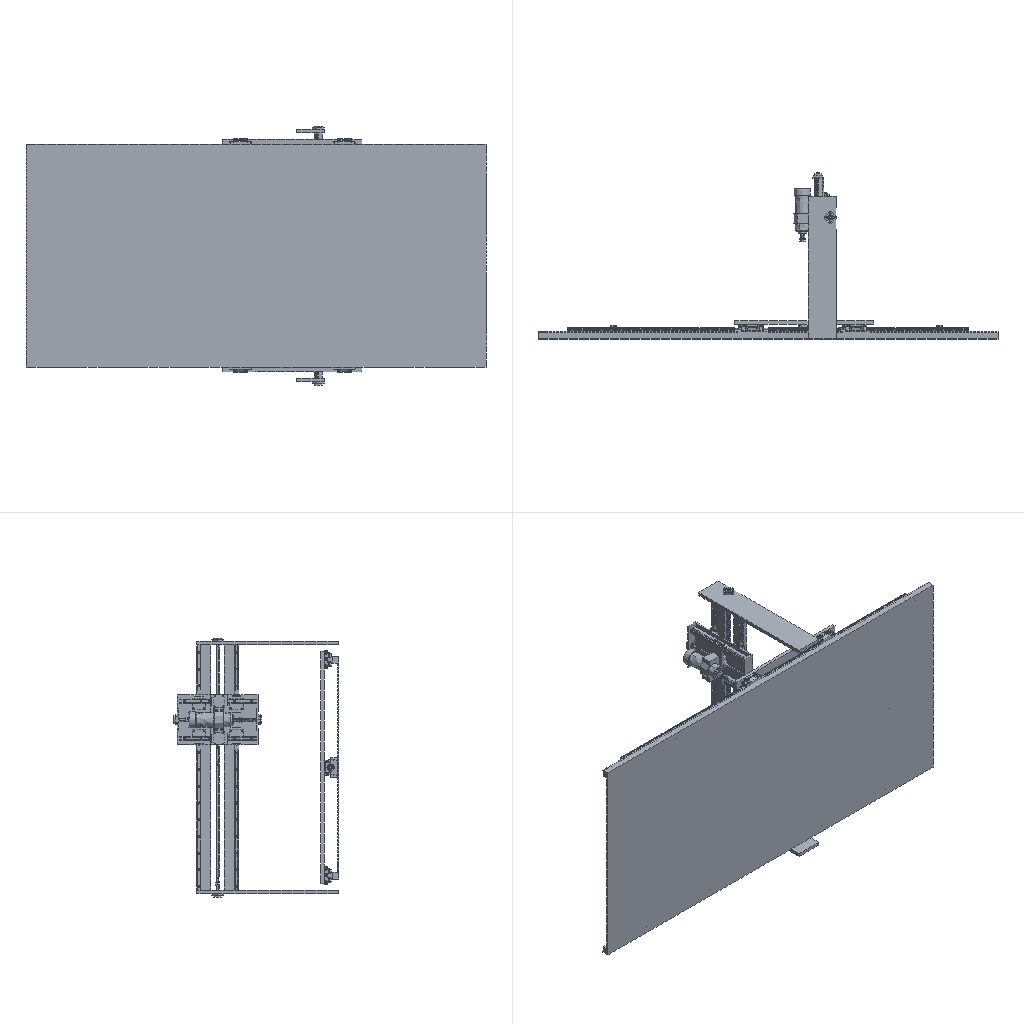Simulation study | ansys workbench
Ansys APDL input file, long lists of numbers shortened:
/batch
/config,noeldb,1     ! force off writing results to database
*get,_wallstrt,active,,time,wall
! ANSYS input file written by Workbench version 2022 R1
! File used for geometry attach: F:\ansys（分析文件汇总)\石材数控线距设备关键零部件分析\底板有限元分析.STEP
/title,wbnew--____ (D5)
! ****** Begin Custom Load Command Snippet ******
/COM, ACT Extensions:
/COM,     LSDYNA, 2021.1
/COM,
! ****** End   Custom Load Command Snippet ******
*DIM,_wb_ProjectScratch_dir,string,248
_wb_ProjectScratch_dir(1) = 'C:\Users\Administrator\AppData\Local\Temp\WB_Administrator_1940_2\_ProjectScratch\Scr49AF\'
*DIM,_wb_SolverFiles_dir,string,248
_wb_SolverFiles_dir(1) = 'C:\Users\Administrator\AppData\Local\Temp\WB_Administrator_1940_2\wbnew_files\dp0\SYS-1\MECH\'
*DIM,_wb_userfiles_dir,string,248
_wb_userfiles_dir(1) = 'C:\Users\Administrator\AppData\Local\Temp\WB_Administrator_1940_2\wbnew_files\user_files\'
/com,--- Data in consistent NMM units. See Solving Units in the help system for more information.
/units,MPA
/nopr
/wb,file,start              !  signify a WB generated input file
/prep7
! Turn off shape checking because checks already performed inside WB mesher.
! See help system for more information.
SHPP,OFF,,NOWARN
/nolist
etcon,set             ! allow ANSYS to choose best KEYOP's for 180x elements, resets any applicable keyopt to MAPDL defaults
/com,*********** Nodes for the whole assembly ***********
nblock,3,,8471
(1i9,3e20.9e3)
        1     3.970000000E+02     2.479000000E+01     8.250000000E+02
! (7700 more lines like these left out)
-1
/wb,elem,start            !  set before creation of elements
/com,*********** Elements for Body 1 "_______-FreeParts|NONE" ***********
et,1,187
eblock,19,solid,,3637
(19i9)
        1        1        1        1        0        0        0        0       10        0        1      804     1262     1046     1255     5874     7115     5872     5873
! (7273 more lines like these left out)
-1
/wb,elem,end               !  done creating elements
/com,*********** Send User Defined Coordinate System(s) ***********
csys,0
toffst,273.15,  ! Temperature offset from absolute zero
/com,*********** Set Reference Temperature ***********
tref,22.
/wb,mat,start              !  starting to send materials
/com,*********** Send Materials ***********
Temperature = 'TEMP' ! Temperature
MP,DENS,1,7.85e-09,	! tonne mm^-3
MP,ALPX,1,1.2e-05,	! C^-1
MP,C,1,434000000,	! mm^2 s^-2 C^-1
MP,KXX,1,60.5,	! tonne mm s^-3 C^-1
MP,RSVX,1,0.00017,	! ohm mm
MP,EX,1,200000,	! tonne s^-2 mm^-1
MP,NUXY,1,0.3,
MP,MURX,1,10000,
/wb,mat,end                !  done sending materials
!************************* Model Summary ********************
!_______-FreeParts|NONE,	结构钢,	matid,	1
!************************* End Model Summary ********************
! get the diagonal of the bounding box. Needed later for other things
*get,_xmin,node,,mnloc,x
*get,_ymin,node,,mnloc,y
*get,_zmin,node,,mnloc,z
*get,_xmax,node,,mxloc,x
*get,_ymax,node,,mxloc,y
*get,_zmax,node,,mxloc,z
_ASMDIAG=(_xmax-_xmin)*(_xmax-_xmin)+(_ymax-_ymin)*(_ymax-_ymin)+(_zmax-_zmin)*(_zmax-_zmin)
_ASMDIAG=SQRT(_ASMDIAG)
/wb,contact,start          !  starting to send contact
/wb,contact,end            !  done creating contacts
/golist
/wb,load,start             !  starting to send loads
/com,*********** Fixed Supports ***********
CMBLOCK,_FIXEDSU,NODE,     1175
(8i10)
       349       350       351       352       353       354       355       356
! (146 more lines like these left out)
cmsel,s,_FIXEDSU
d,all,all
nsel,all
/com,*********** Define Force Using Surface Effect Elements ***********
local,12,0,0.,0.,0.,0.,0.,0.
csys,0
et,2,154
eblock,10,,,782
(15i9)
     6272        2        2        2       12      861     1043      990      990     5982     6910      990     5980
! (781 more lines like these left out)
-1
esel,s,type,,2
keyop,2,2,1                ! Apply load in local coordinate system
keyop,2,7,1                ! Use original area so load is constant in large deformation
esel,all
/gst,on,on
fini
*get,_numnode,node,0,count
*get,_numelem,elem,0,count
*get, _MAXELEMNUM, elem, 0, NUM, MAX
*get, _MAXNODENUM, node, 0, NUM, MAX
*get, _MAXELEMTYPE, etyp, 0, NUM, MAX
*get, _MAXREALCONST, real, 0, NUM, MAX
/go
/wb,load,end               !  done creating loads
/com,--- Number of total nodes = %_numnode%
/com,--- Number of contact elements = 782
/com,--- Number of spring elements = 0
/com,--- Number of bearing elements = 0
/com,--- Number of solid elements = 3637
/com,--- Number of condensed parts = 0
/com,--- Number of total elements = %_numelem%
*get,_wallbsol,active,,time,wall
/com,****************************************************************************
/com,*************************    SOLUTION       ********************************
/com,****************************************************************************
/solu
antype,0                   ! static analysis
_thickRatio=  0     ! Ratio of thick parts in the model
eqsl,sparse,,,,,1
cntr,print,1               ! print out contact info and also make no initial contact an error
dmpoption,emat,no             ! Don't combine emat file for DANSYS
dmpoption,esav,no             ! Don't combine esav file for DANSYS
nldiag,cont,iter           ! print out contact info each equilibrium iteration
rescontrol,,none                 ! Do not keep any restart files
/com,****************************************************
/com,******************* SOLVE FOR LS 1 OF 1 ****************
esel,s,type,,2
nsle
sfe,all,1,pres,1,0.
sfe,all,2,pres,1,-381.65
sfe,all,3,pres,1,0.
nsel,all
esel,all
/nopr
/gopr
nsub,1,1,1
time,1.
outres,erase
outres,all,none
outres,nsol,all,
outres,rsol,all
outres,eangl,all
outres,etmp,all
outres,veng,all
outres,strs,all,
outres,epel,all,
outres,eppl,all,
outres,cont,all,
! *********** WB SOLVE COMMAND ***********
! check interactive state
*get,ANSINTER_,active,,int
*if,ANSINTER_,ne,0,then
/eof
*endif
solve
/com *************** Write FE CONNECTORS *********
CEWRITE,file,ce,,INTE
/com,****************************************************
/com,*************** FINISHED SOLVE FOR LS 1 *************
*get,_wallasol,active,,time,wall
/nopr
*get,_numnode,node,0,count
*get,_numelem,elem,0,count
*get, _MAXELEMNUM, elem, 0, NUM, MAX
*get, _MAXNODENUM, node, 0, NUM, MAX,,,INTERNAL
*get, _MAXELEMTYPE, etyp, 0, NUM, MAX
*get, _MAXREALCONST, real, 0, NUM, MAX
/gopr
/post1
xmlo,ENCODING,ISO-8859-1
xmlo,parm
/xml,parm,xml
fini
/gopr
*get,_walldone,active,,time,wall
_preptime=(_wallbsol-_wallstrt)*3600
_solvtime=(_wallasol-_wallbsol)*3600
_posttime=(_walldone-_wallasol)*3600
_totaltim=(_walldone-_wallstrt)*3600
*get,_dlbratio,active,0,solu,dlbr
*get,_combtime,active,0,solu,comb
*get,_ssmode,active,0,solu,ssmm
*get,_ndofs,active,0,solu,ndof
*get,_sol_end_time,active,0,set,time
*if,_sol_end_time,eq,1.,then
/fclean				!clean distributed files
*endif
/com,--- Total number of nodes = %_numnode%
/com,--- Total number of elements = %_numelem%
/com,--- Element load balance ratio = %_dlbratio%
/com,--- Time to combine distributed files = %_combtime%
/com,--- Sparse memory mode = %_ssmode%
/com,--- Number of DOF = %_ndofs%
/wb,file,end               ! done with WB generated input